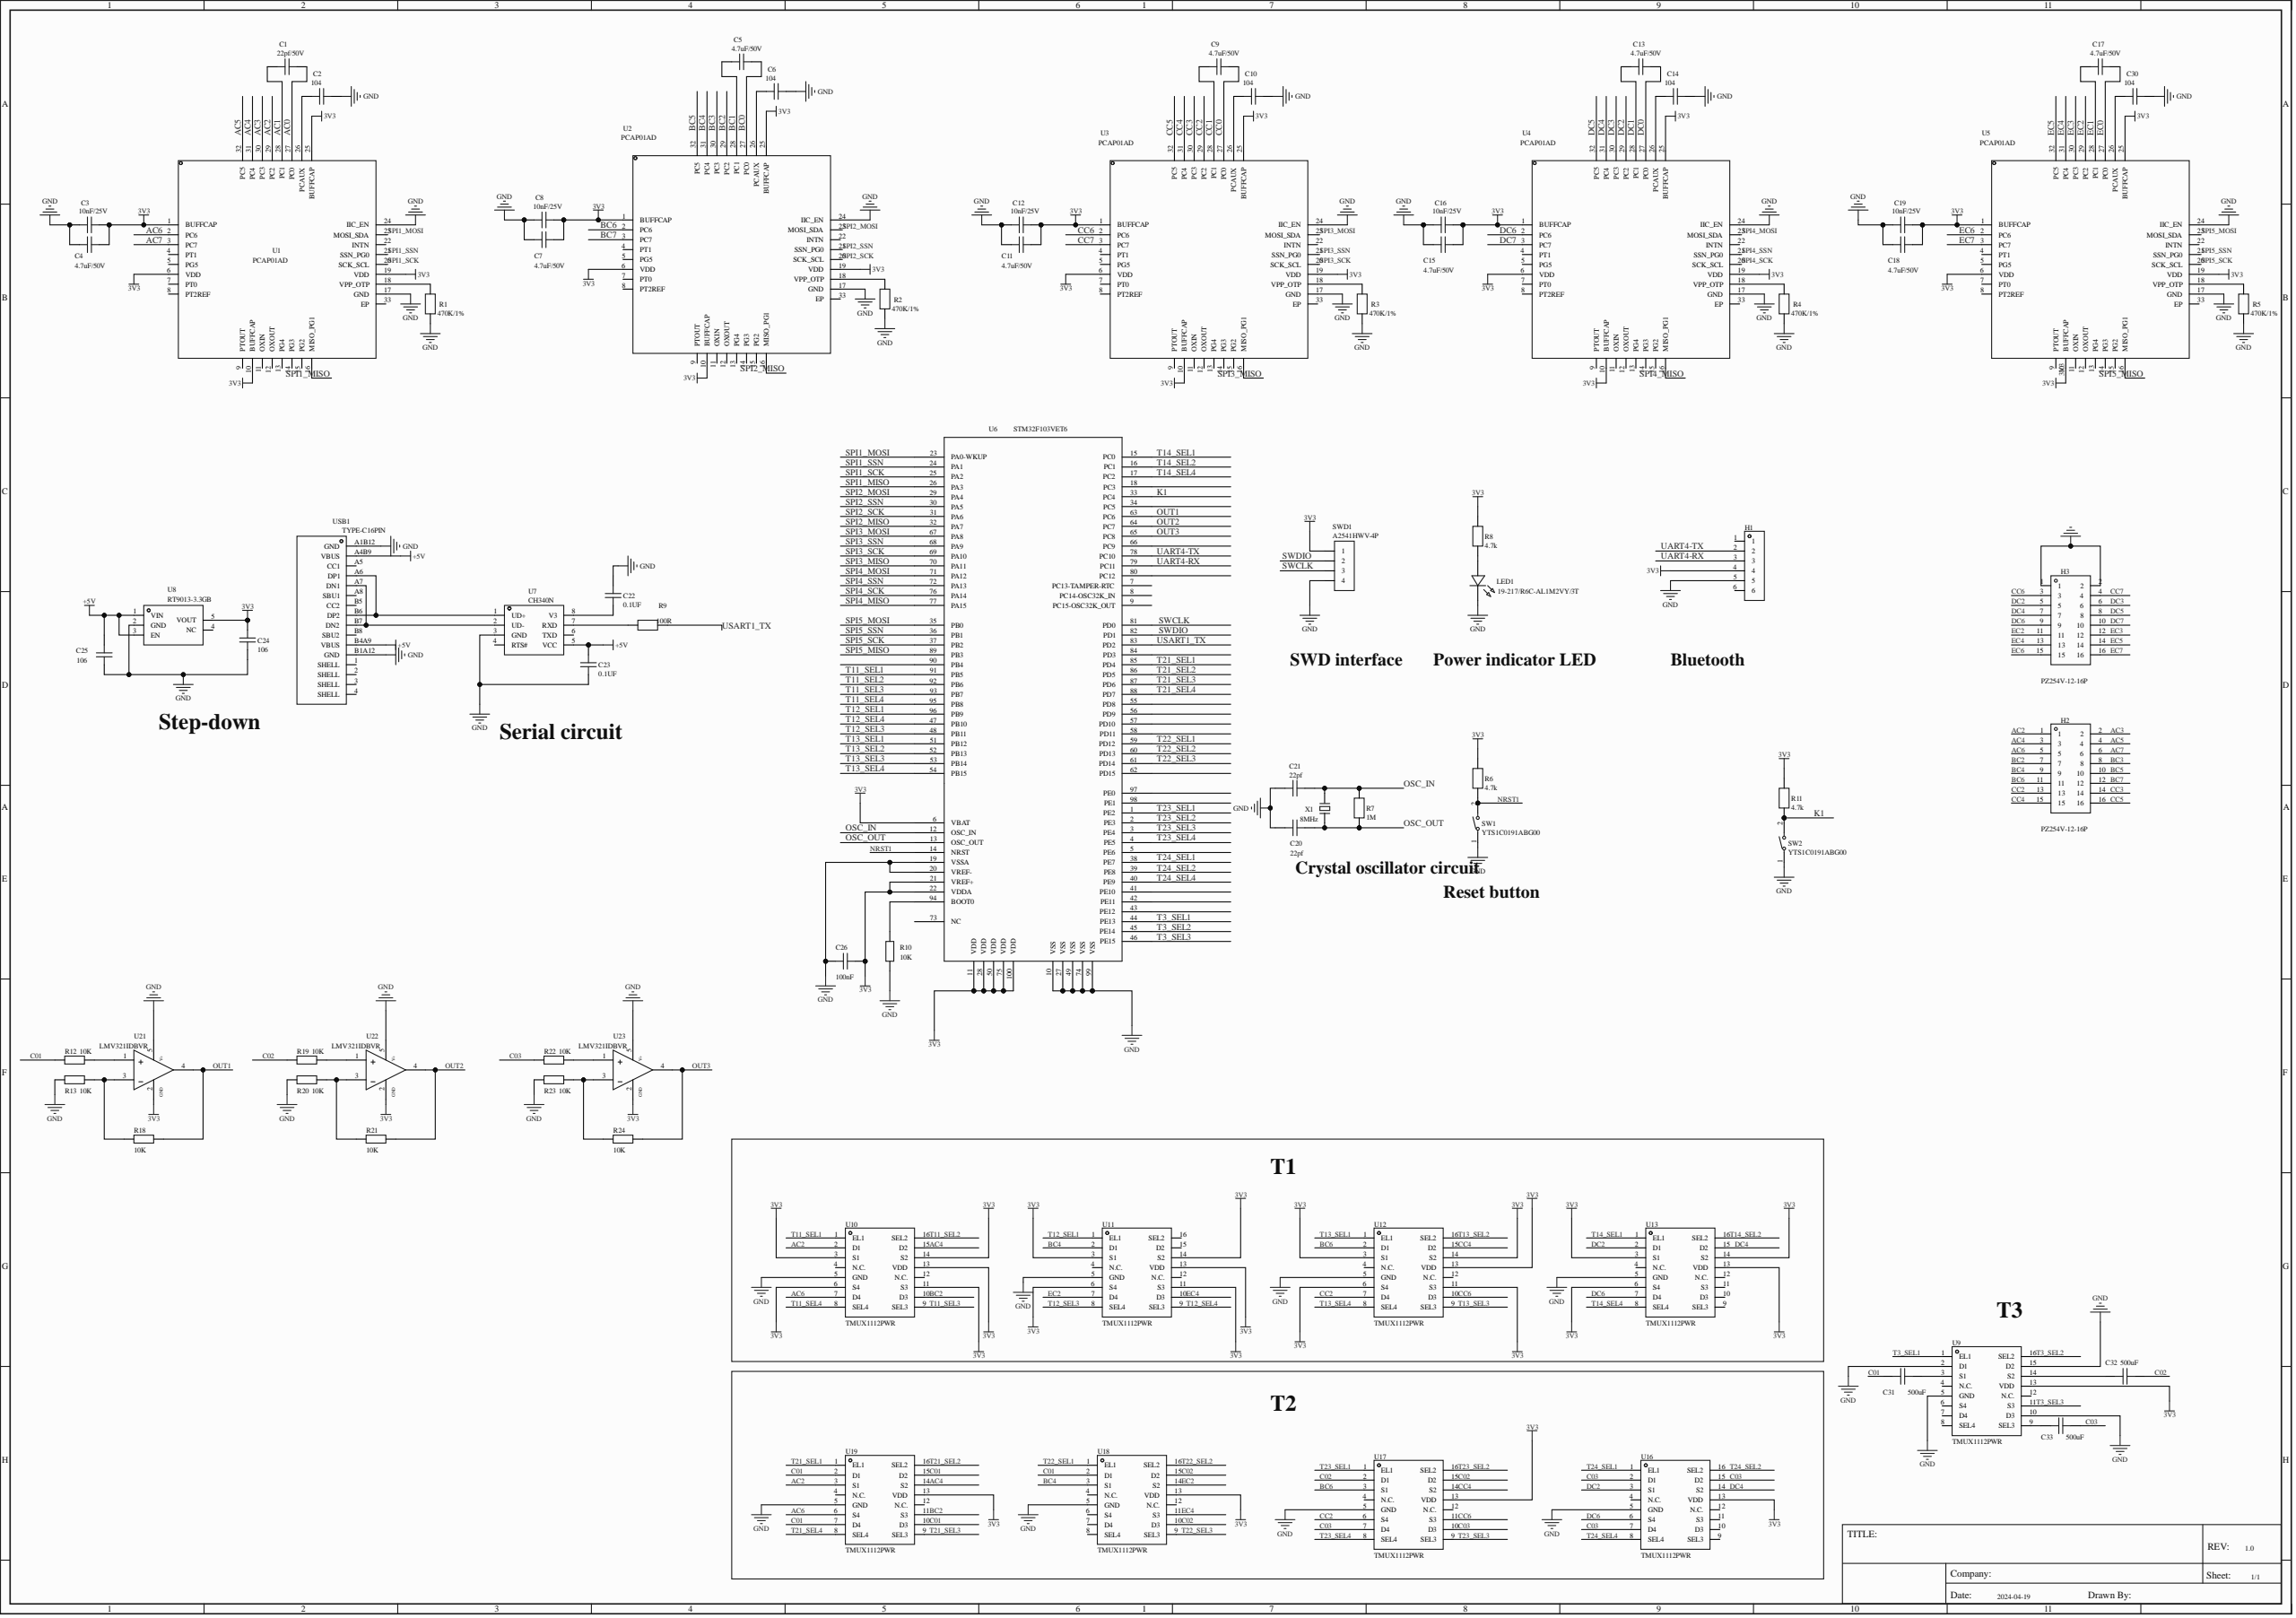Circuit board | Altium Designer | 79 parts | 134 nets
Bill of materials:
Comment,Description,Designator,Footprint,LibRef,Quantity
"22pf/50V","","C1","C0603","4.7uF/50V","1"
"104","","C2, C6, C10, C14, C30","C0603","104","5"
"10nF/25V","","C3, C8, C12, C16, C19","C0603","10nF/25V","5"
"4.7uF/50V","","C4, C5, C7, C9, C11, C13, C15, C17, C18","C0603","4.7uF/50V","9"
"22pf","","C20, C21","C0603","22pf","2"
"0.1UF","","C22, C23","C0603","0.1UF","2"
"106","","C24, C25","C0603","106","2"
"100nF","","C26","C0603","CAP_0603","1"
"500uF","","C31, C32, C33","C0603","CAP_0603","3"
"","","H1","HDR-TH_6P-P2.54-V-F","HDR-F_2.54_1x6P","1"
"PZ254V-12-16P","Pin structure:2x8P;Pitch:2.54mm;Row spacing:2.54mm;Round/square pin:Square pin;Mounting:Through-hole;Number of rows:Double row;Total pin count:16P;Rated current:-;Rated voltage:-;Mating pin length:6mm;Shell height:2.5mm;Tail pin length:3mm;Contact material:Brass;Contact plating:-;Operating temperature:-40℃~+105℃;Color:Black;","H2, H3","HDR-TH_16P-P2.54-V-M-R2-C8-S2.54","PZ254V-12-16P","2"
"19-217/R6C-AL1M2VY/3T","Illumination color:Red;Forward voltage (Vf):1.95V;Power:60mW;Forward current:5mA;Wavelength:617.5nm;Diode configuration:-;Lens color:Colorless transparent lens;Color temperature:-;Viewing angle:120°;Tape packaging:-;Operating temperature:-40℃~+85℃;","LED1","LED0603-RD","19-217/R6C-AL1M2VY/3T","1"
"470K/1%","","R1, R2, R3, R4, R5","R0603","470K/1%","5"
"4.7k","","R6, R8, R11","R0603","4.7k","3"
"1M","","R7","R0603","1M","1"
"100R","","R9","R0603","100R","1"
"10K","","R10, R12, R13, R18, R19, R20, R21, R22, R23, R24","R0603","Res_0603","10"
"YTS1C0191ABG00","","SW1, SW2","SW-SMD_L6.0-W4.0-LS7.2","YTS1C0191ABG00","2"
"A2541HWV-4P","Socket structure:1x4P;Pitch:2.54mm;Row spacing:-;Round/square hole:Square hole;Mounting:Through-hole;Number of rows:Single row;Total hole count:4P;Rated current:3A;Rated voltage:250V;Socket direction:Top;Shell height:8.5mm;Contact material:Brass;Contact plating:Gold;Operating temperature:-40℃~+105℃;","SWD1","HDR-TH_4P-P2.54-V_A2541HWV-4P","A2541HWV-4P","1"
"PCAP01AD","Resolution:17-bit;Operating voltage:2.1V~3.6V;Interface type:SPI; I2C;","U1, U2, U3, U4, U5","VQFN-32_L5.0-W5.0-P0.50-TL-EP","PCAP01AD","5"
"STM32F103VET6","CPU core:ARM-M3;Max CPU frequency:72MHz;Application field:-;","U6","LQFP-100_L14.0-W14.0-P0.50-LS16.0-BL","STM32F103VET6","1"
"CH340N","","U7","SOP-8_150MIL","CH340N","1"
"RT9013-3.3GB","","U8","SOT-23-5_L2.9-W1.6-P0.94-LS2.8-BL","RT9013-3.3GB","1"
"TMUX1112PWR","Switch circuit:Single-pole single-throw (SPST);Channel count:4;On-resistance (Ron@VCC):4O;","U9, U10, U11, U12, U13, U16, U17, U18, U19","TSSOP-16_L5.0-W4.4-P0.65-LS6.4-TL","TMUX1112PWR","9"
"LMV321IDBVR","Amplifier count:Single;Rail-to-rail:Rail-to-rail output;Gain bandwidth product (GBP):1MHz;Input offset voltage (Vos):7mV;Slew rate (SR):1V/us;Input bias current (Ib):11nA;","U21, U22, U23","SOT-23-5_L3.0-W1.7-P0.95-LS2.8-BR","LMV321IDBVR_C7972","3"
"TYPE-C16PIN","Connector type:Type-C;Protocol standard:USB 3.1;Gender:Female;Mounting:Flat-mount;Contact count:16P;Port count:1;Rated current - power:3A;Operating temperature:-40℃~+85℃;","USB1","USB-C-SMD_TYPE-C16PIN","TYPE-C16PIN","1"
"8MHz","","X1","SMD322522","8MHz","1"
Netlist (Protel format):
[
C1
C0603
22pf/50V



]
[
C2
C0603
104



]
[
C3
C0603
10nF/25V



]
[
C4
C0603
4.7uF/50V



]
[
C5
C0603
4.7uF/50V



]
[
C6
C0603
104



]
[
C7
C0603
4.7uF/50V



]
[
C8
C0603
10nF/25V



]
[
C9
C0603
4.7uF/50V



]
[
C10
C0603
104



]
[
C11
C0603
4.7uF/50V



]
[
C12
C0603
10nF/25V



]
[
C13
C0603
4.7uF/50V



]
[
C14
C0603
104



]
[
C15
C0603
4.7uF/50V



]
[
C16
C0603
10nF/25V



]
[
C17
C0603
4.7uF/50V



]
[
C18
C0603
4.7uF/50V



]
[
C19
C0603
10nF/25V



]
[
C20
C0603
22pf



]
[
C21
C0603
22pf



]
[
C22
C0603
0.1UF



]
[
C23
C0603
0.1UF



]
[
C24
C0603
106



]
[
C25
C0603
106



]
[
C26
C0603
100nF



]
[
C30
C0603
104



]
[
C31
C0603
500uF



]
[
C32
C0603
500uF



]
[
C33
C0603
500uF



]
[
H1
HDR-TH_6P-P2.54-V-F




]
[
H2
HDR-TH_16P-P2.54-V-M-R2-C8-S2.54
PZ254V-12-16P



]
[
H3
HDR-TH_16P-P2.54-V-M-R2-C8-S2.54
PZ254V-12-16P



]
[
LED1
LED0603-RD
19-217/R6C-AL1M2VY/3T



]
[
R1
R0603
470K/1%



]
[
R2
R0603
470K/1%



]
[
R3
R0603
470K/1%



]
[
R4
R0603
470K/1%



]
[
R5
R0603
470K/1%



]
[
R6
R0603
4.7k



]
[
R7
R0603
1M



]
[
R8
R0603
4.7k



]
[
R9
R0603
100R



]
[
R10
R0603
10K



]
[
R11
R0603
4.7k



]
[
R12
R0603
10K



]
[
R13
R0603
10K



]
[
R18
R0603
10K



]
[
R19
R0603
10K



]
[
R20
R0603
10K



]
[
R21
R0603
10K



]
[
R22
R0603
10K



]
[
R23
R0603
10K



]
[
R24
R0603
10K



]
[
SW1
SW-SMD_L6.0-W4.0-LS7.2
YTS1C0191ABG00



]
[
SW2
SW-SMD_L6.0-W4.0-LS7.2
YTS1C0191ABG00



]
[
SWD1
HDR-TH_4P-P2.54-V_A2541HWV-4P
A2541HWV-4P



]
[
U1
VQFN-32_L5.0-W5.0-P0.50-TL-EP
PCAP01AD



]
[
U2
VQFN-32_L5.0-W5.0-P0.50-TL-EP
PCAP01AD



]
[
U3
VQFN-32_L5.0-W5.0-P0.50-TL-EP
PCAP01AD



]
[
U4
VQFN-32_L5.0-W5.0-P0.50-TL-EP
PCAP01AD



]
[
U5
VQFN-32_L5.0-W5.0-P0.50-TL-EP
PCAP01AD



]
[
U6
LQFP-100_L14.0-W14.0-P0.50-LS16.0-BL
STM32F103VET6



]
[
U7
SOP-8_150MIL
CH340N



]
[
U8
SOT-23-5_L2.9-W1.6-P0.94-LS2.8-BL
RT9013-3.3GB



]
[
U9
TSSOP-16_L5.0-W4.4-P0.65-LS6.4-TL
TMUX1112PWR



]
[
U10
TSSOP-16_L5.0-W4.4-P0.65-LS6.4-TL
TMUX1112PWR



]
[
U11
TSSOP-16_L5.0-W4.4-P0.65-LS6.4-TL
TMUX1112PWR



]
[
U12
TSSOP-16_L5.0-W4.4-P0.65-LS6.4-TL
TMUX1112PWR



]
[
U13
TSSOP-16_L5.0-W4.4-P0.65-LS6.4-TL
TMUX1112PWR



]
[
U16
TSSOP-16_L5.0-W4.4-P0.65-LS6.4-TL
TMUX1112PWR



]
[
U17
TSSOP-16_L5.0-W4.4-P0.65-LS6.4-TL
TMUX1112PWR



]
[
U18
TSSOP-16_L5.0-W4.4-P0.65-LS6.4-TL
TMUX1112PWR



]
[
U19
TSSOP-16_L5.0-W4.4-P0.65-LS6.4-TL
TMUX1112PWR



]
[
U21
SOT-23-5_L3.0-W1.7-P0.95-LS2.8-BR
LMV321IDBVR



]
[
U22
SOT-23-5_L3.0-W1.7-P0.95-LS2.8-BR
LMV321IDBVR



]
[
U23
SOT-23-5_L3.0-W1.7-P0.95-LS2.8-BR
LMV321IDBVR



]
[
USB1
USB-C-SMD_TYPE-C16PIN
TYPE-C16PIN



]
[
X1
SMD322522
8MHz



]
(
USART1_TX
R9-2
U6-83
)
(
UART4-TX
H1-2
U6-78
)
(
UART4-RX
H1-3
U6-79
)
(
T24_SEL4
U6-40
U16-8
)
(
T24_SEL2
U6-39
U16-16
)
(
T24_SEL1
U6-38
U16-1
)
(
T23_SEL4
U6-4
U17-8
)
(
T23_SEL3
U6-3
U17-9
)
(
T23_SEL2
U6-2
U17-16
)
(
T23_SEL1
U6-1
U17-1
)
(
T22_SEL3
U6-61
U18-9
)
(
T22_SEL2
U6-60
U18-16
)
(
T22_SEL1
U6-59
U18-1
)
(
T21_SEL4
U6-88
U19-8
)
(
T21_SEL3
U6-87
U19-9
)
(
T21_SEL2
U6-86
U19-16
)
(
T21_SEL1
U6-85
U19-1
)
(
T14_SEL4
U6-17
U13-8
)
(
T14_SEL2
U6-16
U13-16
)
(
T14_SEL1
U6-15
U13-1
)
(
T13_SEL4
U6-54
U12-8
)
(
T13_SEL3
U6-53
U12-9
)
(
T13_SEL2
U6-52
U12-16
)
(
T13_SEL1
U6-51
U12-1
)
(
T12_SEL4
U6-47
U11-9
)
(
T12_SEL3
U6-48
U11-8
)
(
T12_SEL1
U6-96
U11-1
)
(
T11_SEL4
U6-95
U10-8
)
(
T11_SEL3
U6-93
U10-9
)
(
T11_SEL2
U6-92
U10-16
)
(
T11_SEL1
U6-91
U10-1
)
(
T3_SEL3
U6-46
U9-11
)
(
T3_SEL2
U6-45
U9-16
)
(
T3_SEL1
U6-44
U9-1
)
(
SWDIO
SWD1-2
U6-82
)
(
SWCLK
SWD1-3
U6-81
)
(
SPI5_SSN
U5-21
U6-36
)
(
SPI5_SCK
U5-20
U6-37
)
(
SPI5_MOSI
U5-23
U6-35
)
(
SPI5_MISO
U5-16
U6-89
)
(
SPI4_SSN
U4-21
U6-72
)
(
SPI4_SCK
U4-20
U6-76
)
(
SPI4_MOSI
U4-23
U6-71
)
(
SPI4_MISO
U4-16
U6-77
)
(
SPI3_SSN
U3-21
U6-68
)
(
SPI3_SCK
U3-20
U6-69
)
(
SPI3_MOSI
U3-23
U6-67
)
(
SPI3_MISO
U3-16
U6-70
)
(
SPI2_SSN
U2-21
U6-30
)
(
SPI2_SCK
U2-20
U6-31
)
(
SPI2_MOSI
U2-23
U6-29
)
(
SPI2_MISO
U2-16
U6-32
)
(
SPI1_SSN
U1-21
U6-24
)
(
SPI1_SCK
U1-20
U6-25
)
(
SPI1_MOSI
U1-23
U6-23
)
(
SPI1_MISO
U1-16
U6-26
)
(
OUT3
R24-2
U6-65
U23-4
)
(
OUT2
R21-2
U6-64
U22-4
)
(
OUT1
R18-2
U6-63
U21-4
)
(
OSC_OUT
C20-2
R7-1
U6-13
X1-1
)
(
OSC_IN
C21-2
R7-2
U6-12
X1-2
)
(
NRST1
R6-1
SW1-2
U6-14
)
(
NetU7_2
U7-2
USB1-A7
USB1-B7
)
(
NetU7_1
U7-1
USB1-A6
USB1-B6
)
(
NetR23_2
R23-2
R24-1
U23-3
)
(
NetR22_2
R22-2
U23-1
)
(
NetR20_2
R20-2
R21-1
U22-3
)
(
NetR19_2
R19-2
U22-1
)
(
NetR13_2
R13-2
R18-1
U21-3
)
(
NetR12_2
R12-2
U21-1
)
(
NetR10_1
R10-1
U6-94
)
(
NetR9_1
R9-1
U7-7
)
(
NetR5_2
R5-2
U5-18
)
(
NetR4_2
R4-2
U4-18
)
(
NetR3_2
R3-2
U3-18
)
(
NetR2_2
R2-2
U2-18
)
(
NetR1_2
R1-2
U1-18
)
(
NetLED1_1
LED1-1
R8-1
)
(
NetC33_2
C33-2
U9-9
)
(
NetC32_2
C32-2
U9-14
)
(
NetC31_1
C31-1
U9-3
)
(
NetC30_1
C30-1
U5-26
)
(
NetC22_1
C22-1
U7-8
)
(
NetC14_1
C14-1
U4-26
)
(
NetC10_1
C10-1
U3-26
)
(
NetC6_1
C6-1
U2-26
)
(
NetC2_1
C2-1
U1-26
)
(
K1
R11-1
SW2-2
U6-33
)
(
GND
C2-2
C3-1
C4-1
C6-2
C7-1
C8-1
C10-2
C11-1
C12-1
C14-2
C15-1
C16-1
C18-1
C19-1
C20-1
C21-1
C22-2
C23-1
C24-1
C25-1
C26-1
C30-2
H1-5
H3-1
H3-2
LED1-2
R1-1
R2-1
R3-1
R4-1
R5-1
R10-2
R13-1
R20-1
R23-1
SW1-1
SW2-1
SWD1-4
U1-17
U1-24
U2-17
U2-24
U3-17
U3-24
U4-17
U4-24
U5-17
U5-24
U6-10
U6-19
U6-20
U6-27
U6-49
U6-74
U6-99
U7-3
U8-2
U9-2
U9-5
U9-10
U9-15
U10-5
U11-5
U12-5
U13-5
U16-5
U17-5
U18-5
U19-5
U21-5
U22-5
U23-5
USB1-A1B12
USB1-B1A12
)
(
EC7
H3-16
U5-3
)
(
EC6
H3-15
U5-2
)
(
EC5
H3-14
U5-32
)
(
EC4
H3-13
U5-31
U11-10
U18-11
)
(
EC3
H3-12
U5-30
)
(
EC2
H3-11
U5-29
U11-7
U18-14
)
(
EC1
C17-1
U5-28
)
(
EC0
C17-2
U5-27
)
(
DC7
H3-10
U4-3
)
(
DC6
H3-9
U4-2
U13-7
U16-6
)
(
DC5
H3-8
U4-32
)
(
DC4
H3-7
U4-31
U13-15
U16-14
)
(
DC3
H3-6
U4-30
)
(
DC2
H3-5
U4-29
U13-2
U16-3
)
(
DC1
C13-1
U4-28
)
(
DC0
C13-2
U4-27
)
(
CC7
H3-4
U3-3
)
(
CC6
H3-3
U3-2
U12-10
U17-11
)
(
CC5
H2-16
U3-32
)
(
CC4
H2-15
U3-31
U12-15
U17-14
)
(
CC3
H2-14
U3-30
)
(
CC2
H2-13
U3-29
U12-7
U17-6
)
(
CC1
C9-1
U3-28
)
(
CC0
C9-2
U3-27
)
(
C03
C33-1
R22-1
U16-2
U16-7
U16-15
U17-7
U17-10
)
(
C02
C32-1
R19-1
U17-2
U17-15
U18-10
U18-15
)
(
C01
C31-2
R12-1
U18-2
U19-2
U19-7
U19-10
U19-15
)
(
BC7
H2-12
U2-3
)
(
BC6
H2-11
U2-2
U12-2
U17-3
)
(
BC5
H2-10
U2-32
)
(
BC4
H2-9
U2-31
U11-2
U18-3
)
(
BC3
H2-8
U2-30
)
(
BC2
H2-7
U2-29
U10-10
U19-11
)
(
BC1
C5-1
U2-28
)
(
BC0
C5-2
U2-27
)
(
AC7
H2-6
U1-3
)
(
AC6
H2-5
U1-2
U10-7
U19-6
)
(
AC5
H2-4
U1-32
)
(
AC4
H2-3
U1-31
U10-15
U19-14
)
(
AC3
H2-2
U1-30
)
(
AC2
H2-1
U1-29
U10-2
U19-3
)
(
AC1
C1-1
U1-28
)
(
AC0
C1-2
U1-27
)
(
+5V
C23-2
C25-2
U7-5
U8-1
U8-3
USB1-A4B9
USB1-B4A9
)
(
3V3
C3-2
C4-2
C7-2
C8-2
C11-2
C12-2
C15-2
C16-2
C18-2
C19-2
C24-2
C26-2
H1-4
R6-2
R8-2
R11-2
SWD1-1
U1-1
U1-6
U1-10
U1-19
U1-25
U2-1
U2-6
U2-10
U2-19
U2-25
U3-1
U3-6
U3-10
U3-19
U3-25
U4-1
U4-6
U4-10
U4-19
U4-25
U5-1
U5-6
U5-10
U5-19
U5-25
U6-6
U6-11
U6-21
U6-22
U6-28
U6-50
U6-75
U6-100
U8-5
U9-13
U10-3
U10-6
U10-11
U10-13
U10-14
U11-3
U11-6
U11-11
U11-13
U11-14
U12-3
U12-6
U12-11
U12-13
U12-14
U13-3
U13-6
U13-13
U13-14
U16-13
U17-13
U18-13
U19-13
U21-2
U22-2
U23-2
)